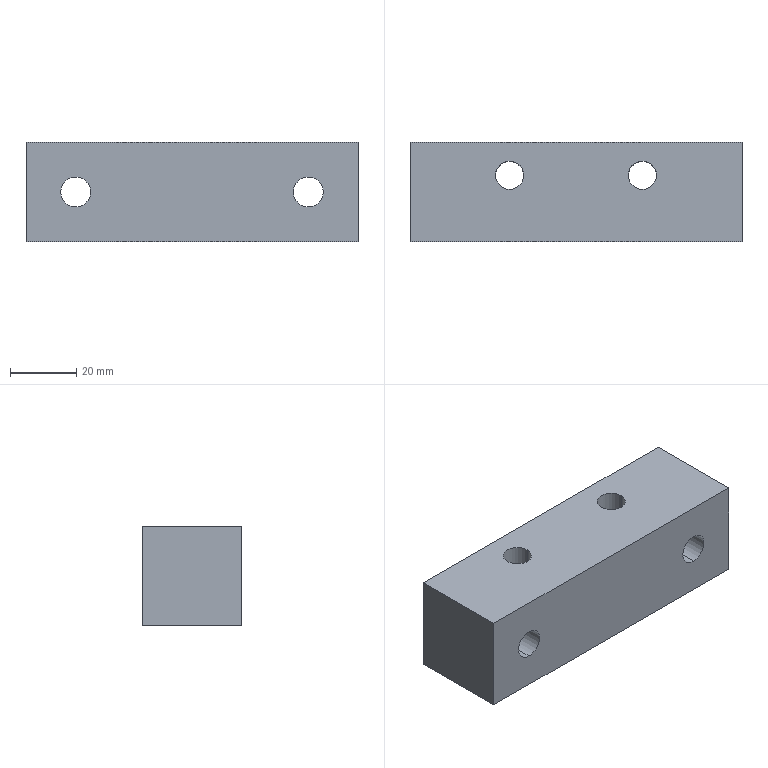Part | SolidWorks | features HoleWzd 2, Extrusion 1 | 1 solid | 20 faces | box 100 x 30 x 30 mm | volume 78254 mm3 | cylinder 12 | plane 8 | commonest cylinder face diameters 8.5 x4 9 x4 15 x4
STEP:
#1=CARTESIAN_POINT('',(-24.25,5.,0.));
#2=VERTEX_POINT('',#1);
#3=CARTESIAN_POINT('',(-15.75,5.,0.));
#4=VERTEX_POINT('',#3);
#5=CARTESIAN_POINT('',(-20.,5.,0.));
#6=DIRECTION('',(0.,0.,1.));
#7=DIRECTION('',(1.,0.,0.));
#8=AXIS2_PLACEMENT_3D('',#5,#6,#7);
#9=CIRCLE('',#8,4.25);
#10=EDGE_CURVE('',#2,#4,#9,.T.);
#11=ORIENTED_EDGE('',*,*,#10,.F.);
#12=CARTESIAN_POINT('',(-24.25,5.,30.));
#13=VERTEX_POINT('',#12);
#14=CARTESIAN_POINT('',(-24.25,5.,30.));
#15=DIRECTION('',(0.,0.,1.));
#16=VECTOR('',#15,1000.);
#17=LINE('',#14,#16);
#18=EDGE_CURVE('',#2,#13,#17,.T.);
#19=ORIENTED_EDGE('',*,*,#18,.T.);
#20=CARTESIAN_POINT('',(-15.75,5.,30.));
#21=VERTEX_POINT('',#20);
#22=CARTESIAN_POINT('',(-20.,5.,30.));
#23=DIRECTION('',(0.,0.,1.));
#24=DIRECTION('',(1.,0.,0.));
#25=AXIS2_PLACEMENT_3D('',#22,#23,#24);
#26=CIRCLE('',#25,4.25);
#27=EDGE_CURVE('',#13,#21,#26,.T.);
#28=ORIENTED_EDGE('',*,*,#27,.T.);
#29=CARTESIAN_POINT('',(-15.75,5.,30.));
#30=DIRECTION('',(0.,0.,1.));
#31=VECTOR('',#30,1000.);
#32=LINE('',#29,#31);
#33=EDGE_CURVE('',#4,#21,#32,.T.);
#34=ORIENTED_EDGE('',*,*,#33,.F.);
#35=EDGE_LOOP('',(#11,#19,#28,#34));
#36=FACE_OUTER_BOUND('',#35,.T.);
#37=CARTESIAN_POINT('',(-20.,5.,30.));
#38=DIRECTION('',(0.,0.,1.));
#39=DIRECTION('',(1.,0.,0.));
#40=AXIS2_PLACEMENT_3D('',#37,#38,#39);
#41=CYLINDRICAL_SURFACE('',#40,4.25);
#42=ADVANCED_FACE('',(#36),#41,.F.);
#43=CARTESIAN_POINT('',(15.75,5.,0.));
#44=VERTEX_POINT('',#43);
#45=CARTESIAN_POINT('',(24.25,5.,0.));
#46=VERTEX_POINT('',#45);
#47=CARTESIAN_POINT('',(20.,5.,0.));
#48=DIRECTION('',(0.,0.,1.));
#49=DIRECTION('',(1.,0.,0.));
#50=AXIS2_PLACEMENT_3D('',#47,#48,#49);
#51=CIRCLE('',#50,4.25);
#52=EDGE_CURVE('',#44,#46,#51,.T.);
#53=ORIENTED_EDGE('',*,*,#52,.F.);
#54=CARTESIAN_POINT('',(15.75,5.,30.));
#55=VERTEX_POINT('',#54);
#56=CARTESIAN_POINT('',(15.75,5.,30.));
#57=DIRECTION('',(0.,0.,1.));
#58=VECTOR('',#57,1000.);
#59=LINE('',#56,#58);
#60=EDGE_CURVE('',#44,#55,#59,.T.);
#61=ORIENTED_EDGE('',*,*,#60,.T.);
#62=CARTESIAN_POINT('',(24.25,5.,30.));
#63=VERTEX_POINT('',#62);
#64=CARTESIAN_POINT('',(20.,5.,30.));
#65=DIRECTION('',(0.,0.,1.));
#66=DIRECTION('',(1.,0.,0.));
#67=AXIS2_PLACEMENT_3D('',#64,#65,#66);
#68=CIRCLE('',#67,4.25);
#69=EDGE_CURVE('',#55,#63,#68,.T.);
#70=ORIENTED_EDGE('',*,*,#69,.T.);
#71=CARTESIAN_POINT('',(24.25,5.,30.));
#72=DIRECTION('',(0.,0.,1.));
#73=VECTOR('',#72,1000.);
#74=LINE('',#71,#73);
#75=EDGE_CURVE('',#46,#63,#74,.T.);
#76=ORIENTED_EDGE('',*,*,#75,.F.);
#77=EDGE_LOOP('',(#53,#61,#70,#76));
#78=FACE_OUTER_BOUND('',#77,.T.);
#79=CARTESIAN_POINT('',(20.,5.,30.));
#80=DIRECTION('',(0.,0.,1.));
#81=DIRECTION('',(1.,0.,0.));
#82=AXIS2_PLACEMENT_3D('',#79,#80,#81);
#83=CYLINDRICAL_SURFACE('',#82,4.25);
#84=ADVANCED_FACE('',(#78),#83,.F.);
#85=CARTESIAN_POINT('',(-35.,-5.,7.5));
#86=VERTEX_POINT('',#85);
#87=CARTESIAN_POINT('',(-35.,-5.,22.5));
#88=VERTEX_POINT('',#87);
#89=CARTESIAN_POINT('',(-35.,-5.,15.));
#90=DIRECTION('',(0.,1.,0.));
#91=DIRECTION('',(0.,0.,1.));
#92=AXIS2_PLACEMENT_3D('',#89,#90,#91);
#93=CIRCLE('',#92,7.5);
#94=EDGE_CURVE('',#86,#88,#93,.T.);
#95=ORIENTED_EDGE('',*,*,#94,.F.);
#96=CARTESIAN_POINT('',(-35.,15.,7.5));
#97=VERTEX_POINT('',#96);
#98=CARTESIAN_POINT('',(-35.,15.,7.5));
#99=DIRECTION('',(0.,1.,0.));
#100=VECTOR('',#99,1000.);
#101=LINE('',#98,#100);
#102=EDGE_CURVE('',#86,#97,#101,.T.);
#103=ORIENTED_EDGE('',*,*,#102,.T.);
#104=CARTESIAN_POINT('',(-35.,15.,22.5));
#105=VERTEX_POINT('',#104);
#106=CARTESIAN_POINT('',(-35.,15.,15.));
#107=DIRECTION('',(0.,1.,0.));
#108=DIRECTION('',(0.,0.,1.));
#109=AXIS2_PLACEMENT_3D('',#106,#107,#108);
#110=CIRCLE('',#109,7.5);
#111=EDGE_CURVE('',#97,#105,#110,.T.);
#112=ORIENTED_EDGE('',*,*,#111,.T.);
#113=CARTESIAN_POINT('',(-35.,15.,22.5));
#114=DIRECTION('',(0.,1.,0.));
#115=VECTOR('',#114,1000.);
#116=LINE('',#113,#115);
#117=EDGE_CURVE('',#88,#105,#116,.T.);
#118=ORIENTED_EDGE('',*,*,#117,.F.);
#119=EDGE_LOOP('',(#95,#103,#112,#118));
#120=FACE_OUTER_BOUND('',#119,.T.);
#121=CARTESIAN_POINT('',(-35.,15.,15.));
#122=DIRECTION('',(0.,1.,0.));
#123=DIRECTION('',(0.,0.,1.));
#124=AXIS2_PLACEMENT_3D('',#121,#122,#123);
#125=CYLINDRICAL_SURFACE('',#124,7.5);
#126=ADVANCED_FACE('',(#120),#125,.F.);
#127=CARTESIAN_POINT('',(-35.,-15.,10.5));
#128=VERTEX_POINT('',#127);
#129=CARTESIAN_POINT('',(-35.,-15.,19.5));
#130=VERTEX_POINT('',#129);
#131=CARTESIAN_POINT('',(-35.,-15.,15.));
#132=DIRECTION('',(0.,1.,0.));
#133=DIRECTION('',(0.,0.,1.));
#134=AXIS2_PLACEMENT_3D('',#131,#132,#133);
#135=CIRCLE('',#134,4.5);
#136=EDGE_CURVE('',#128,#130,#135,.T.);
#137=ORIENTED_EDGE('',*,*,#136,.F.);
#138=CARTESIAN_POINT('',(-35.,-5.,10.5));
#139=VERTEX_POINT('',#138);
#140=CARTESIAN_POINT('',(-35.,15.,10.5));
#141=DIRECTION('',(0.,1.,0.));
#142=VECTOR('',#141,1000.);
#143=LINE('',#140,#142);
#144=EDGE_CURVE('',#128,#139,#143,.T.);
#145=ORIENTED_EDGE('',*,*,#144,.T.);
#146=CARTESIAN_POINT('',(-35.,-5.,19.5));
#147=VERTEX_POINT('',#146);
#148=CARTESIAN_POINT('',(-35.,-5.,15.));
#149=DIRECTION('',(0.,1.,0.));
#150=DIRECTION('',(0.,0.,1.));
#151=AXIS2_PLACEMENT_3D('',#148,#149,#150);
#152=CIRCLE('',#151,4.5);
#153=EDGE_CURVE('',#139,#147,#152,.T.);
#154=ORIENTED_EDGE('',*,*,#153,.T.);
#155=CARTESIAN_POINT('',(-35.,15.,19.5));
#156=DIRECTION('',(0.,1.,0.));
#157=VECTOR('',#156,1000.);
#158=LINE('',#155,#157);
#159=EDGE_CURVE('',#130,#147,#158,.T.);
#160=ORIENTED_EDGE('',*,*,#159,.F.);
#161=EDGE_LOOP('',(#137,#145,#154,#160));
#162=FACE_OUTER_BOUND('',#161,.T.);
#163=CARTESIAN_POINT('',(-35.,15.,15.));
#164=DIRECTION('',(0.,1.,0.));
#165=DIRECTION('',(0.,0.,1.));
#166=AXIS2_PLACEMENT_3D('',#163,#164,#165);
#167=CYLINDRICAL_SURFACE('',#166,4.5);
#168=ADVANCED_FACE('',(#162),#167,.F.);
#169=CARTESIAN_POINT('',(35.,-5.,7.5));
#170=VERTEX_POINT('',#169);
#171=CARTESIAN_POINT('',(35.,-5.,22.5));
#172=VERTEX_POINT('',#171);
#173=CARTESIAN_POINT('',(35.,-5.,15.));
#174=DIRECTION('',(0.,1.,0.));
#175=DIRECTION('',(0.,0.,1.));
#176=AXIS2_PLACEMENT_3D('',#173,#174,#175);
#177=CIRCLE('',#176,7.5);
#178=EDGE_CURVE('',#170,#172,#177,.T.);
#179=ORIENTED_EDGE('',*,*,#178,.F.);
#180=CARTESIAN_POINT('',(35.,15.,7.5));
#181=VERTEX_POINT('',#180);
#182=CARTESIAN_POINT('',(35.,15.,7.5));
#183=DIRECTION('',(0.,1.,0.));
#184=VECTOR('',#183,1000.);
#185=LINE('',#182,#184);
#186=EDGE_CURVE('',#170,#181,#185,.T.);
#187=ORIENTED_EDGE('',*,*,#186,.T.);
#188=CARTESIAN_POINT('',(35.,15.,22.5));
#189=VERTEX_POINT('',#188);
#190=CARTESIAN_POINT('',(35.,15.,15.));
#191=DIRECTION('',(0.,1.,0.));
#192=DIRECTION('',(0.,0.,1.));
#193=AXIS2_PLACEMENT_3D('',#190,#191,#192);
#194=CIRCLE('',#193,7.5);
#195=EDGE_CURVE('',#181,#189,#194,.T.);
#196=ORIENTED_EDGE('',*,*,#195,.T.);
#197=CARTESIAN_POINT('',(35.,15.,22.5));
#198=DIRECTION('',(0.,1.,0.));
#199=VECTOR('',#198,1000.);
#200=LINE('',#197,#199);
#201=EDGE_CURVE('',#172,#189,#200,.T.);
#202=ORIENTED_EDGE('',*,*,#201,.F.);
#203=EDGE_LOOP('',(#179,#187,#196,#202));
#204=FACE_OUTER_BOUND('',#203,.T.);
#205=CARTESIAN_POINT('',(35.,15.,15.));
#206=DIRECTION('',(0.,1.,0.));
#207=DIRECTION('',(0.,0.,1.));
#208=AXIS2_PLACEMENT_3D('',#205,#206,#207);
#209=CYLINDRICAL_SURFACE('',#208,7.5);
#210=ADVANCED_FACE('',(#204),#209,.F.);
#211=CARTESIAN_POINT('',(35.,-15.,10.5));
#212=VERTEX_POINT('',#211);
#213=CARTESIAN_POINT('',(35.,-15.,19.5));
#214=VERTEX_POINT('',#213);
#215=CARTESIAN_POINT('',(35.,-15.,15.));
#216=DIRECTION('',(0.,1.,0.));
#217=DIRECTION('',(0.,0.,1.));
#218=AXIS2_PLACEMENT_3D('',#215,#216,#217);
#219=CIRCLE('',#218,4.5);
#220=EDGE_CURVE('',#212,#214,#219,.T.);
#221=ORIENTED_EDGE('',*,*,#220,.F.);
#222=CARTESIAN_POINT('',(35.,-5.,10.5));
#223=VERTEX_POINT('',#222);
#224=CARTESIAN_POINT('',(35.,15.,10.5));
#225=DIRECTION('',(0.,1.,0.));
#226=VECTOR('',#225,1000.);
#227=LINE('',#224,#226);
#228=EDGE_CURVE('',#212,#223,#227,.T.);
#229=ORIENTED_EDGE('',*,*,#228,.T.);
#230=CARTESIAN_POINT('',(35.,-5.,19.5));
#231=VERTEX_POINT('',#230);
#232=CARTESIAN_POINT('',(35.,-5.,15.));
#233=DIRECTION('',(0.,1.,0.));
#234=DIRECTION('',(0.,0.,1.));
#235=AXIS2_PLACEMENT_3D('',#232,#233,#234);
#236=CIRCLE('',#235,4.5);
#237=EDGE_CURVE('',#223,#231,#236,.T.);
#238=ORIENTED_EDGE('',*,*,#237,.T.);
#239=CARTESIAN_POINT('',(35.,15.,19.5));
#240=DIRECTION('',(0.,1.,0.));
#241=VECTOR('',#240,1000.);
#242=LINE('',#239,#241);
#243=EDGE_CURVE('',#214,#231,#242,.T.);
#244=ORIENTED_EDGE('',*,*,#243,.F.);
#245=EDGE_LOOP('',(#221,#229,#238,#244));
#246=FACE_OUTER_BOUND('',#245,.T.);
#247=CARTESIAN_POINT('',(35.,15.,15.));
#248=DIRECTION('',(0.,1.,0.));
#249=DIRECTION('',(0.,0.,1.));
#250=AXIS2_PLACEMENT_3D('',#247,#248,#249);
#251=CYLINDRICAL_SURFACE('',#250,4.5);
#252=ADVANCED_FACE('',(#246),#251,.F.);
#253=CARTESIAN_POINT('',(-35.,15.,15.));
#254=DIRECTION('',(0.,1.,0.));
#255=DIRECTION('',(0.,0.,1.));
#256=AXIS2_PLACEMENT_3D('',#253,#254,#255);
#257=CIRCLE('',#256,7.5);
#258=EDGE_CURVE('',#105,#97,#257,.T.);
#259=ORIENTED_EDGE('',*,*,#258,.F.);
#260=ORIENTED_EDGE('',*,*,#111,.F.);
#261=EDGE_LOOP('',(#259,#260));
#262=FACE_BOUND('',#261,.T.);
#263=CARTESIAN_POINT('',(50.,15.,0.));
#264=VERTEX_POINT('',#263);
#265=CARTESIAN_POINT('',(-50.,15.,0.));
#266=VERTEX_POINT('',#265);
#267=CARTESIAN_POINT('',(-50.,15.,0.));
#268=DIRECTION('',(-1.,0.,0.));
#269=VECTOR('',#268,1000.);
#270=LINE('',#267,#269);
#271=EDGE_CURVE('',#264,#266,#270,.T.);
#272=ORIENTED_EDGE('',*,*,#271,.T.);
#273=CARTESIAN_POINT('',(-50.,15.,30.));
#274=VERTEX_POINT('',#273);
#275=CARTESIAN_POINT('',(-50.,15.,30.));
#276=DIRECTION('',(0.,0.,-1.));
#277=VECTOR('',#276,1000.);
#278=LINE('',#275,#277);
#279=EDGE_CURVE('',#274,#266,#278,.T.);
#280=ORIENTED_EDGE('',*,*,#279,.F.);
#281=CARTESIAN_POINT('',(50.,15.,30.));
#282=VERTEX_POINT('',#281);
#283=CARTESIAN_POINT('',(-50.,15.,30.));
#284=DIRECTION('',(-1.,0.,0.));
#285=VECTOR('',#284,1000.);
#286=LINE('',#283,#285);
#287=EDGE_CURVE('',#282,#274,#286,.T.);
#288=ORIENTED_EDGE('',*,*,#287,.F.);
#289=CARTESIAN_POINT('',(50.,15.,30.));
#290=DIRECTION('',(0.,0.,-1.));
#291=VECTOR('',#290,1000.);
#292=LINE('',#289,#291);
#293=EDGE_CURVE('',#282,#264,#292,.T.);
#294=ORIENTED_EDGE('',*,*,#293,.T.);
#295=EDGE_LOOP('',(#272,#280,#288,#294));
#296=FACE_OUTER_BOUND('',#295,.T.);
#297=CARTESIAN_POINT('',(35.,15.,15.));
#298=DIRECTION('',(0.,1.,0.));
#299=DIRECTION('',(0.,0.,1.));
#300=AXIS2_PLACEMENT_3D('',#297,#298,#299);
#301=CIRCLE('',#300,7.5);
#302=EDGE_CURVE('',#189,#181,#301,.T.);
#303=ORIENTED_EDGE('',*,*,#302,.F.);
#304=ORIENTED_EDGE('',*,*,#195,.F.);
#305=EDGE_LOOP('',(#303,#304));
#306=FACE_BOUND('',#305,.T.);
#307=CARTESIAN_POINT('',(-50.,15.,30.));
#308=DIRECTION('',(0.,-1.,0.));
#309=DIRECTION('',(0.,0.,-1.));
#310=AXIS2_PLACEMENT_3D('',#307,#308,#309);
#311=PLANE('',#310);
#312=ADVANCED_FACE('',(#262,#296,#306),#311,.F.);
#313=CARTESIAN_POINT('',(50.,-15.,0.));
#314=VERTEX_POINT('',#313);
#315=CARTESIAN_POINT('',(50.,15.,0.));
#316=DIRECTION('',(0.,1.,0.));
#317=VECTOR('',#316,1000.);
#318=LINE('',#315,#317);
#319=EDGE_CURVE('',#314,#264,#318,.T.);
#320=ORIENTED_EDGE('',*,*,#319,.T.);
#321=ORIENTED_EDGE('',*,*,#293,.F.);
#322=CARTESIAN_POINT('',(50.,-15.,30.));
#323=VERTEX_POINT('',#322);
#324=CARTESIAN_POINT('',(50.,15.,30.));
#325=DIRECTION('',(0.,1.,0.));
#326=VECTOR('',#325,1000.);
#327=LINE('',#324,#326);
#328=EDGE_CURVE('',#323,#282,#327,.T.);
#329=ORIENTED_EDGE('',*,*,#328,.F.);
#330=CARTESIAN_POINT('',(50.,-15.,30.));
#331=DIRECTION('',(0.,0.,-1.));
#332=VECTOR('',#331,1000.);
#333=LINE('',#330,#332);
#334=EDGE_CURVE('',#323,#314,#333,.T.);
#335=ORIENTED_EDGE('',*,*,#334,.T.);
#336=EDGE_LOOP('',(#320,#321,#329,#335));
#337=FACE_OUTER_BOUND('',#336,.T.);
#338=CARTESIAN_POINT('',(50.,15.,30.));
#339=DIRECTION('',(-1.,0.,0.));
#340=DIRECTION('',(0.,-1.,0.));
#341=AXIS2_PLACEMENT_3D('',#338,#339,#340);
#342=PLANE('',#341);
#343=ADVANCED_FACE('',(#337),#342,.F.);
#344=CARTESIAN_POINT('',(-50.,-15.,0.));
#345=VERTEX_POINT('',#344);
#346=CARTESIAN_POINT('',(-50.,15.,0.));
#347=DIRECTION('',(0.,-1.,0.));
#348=VECTOR('',#347,1000.);
#349=LINE('',#346,#348);
#350=EDGE_CURVE('',#266,#345,#349,.T.);
#351=ORIENTED_EDGE('',*,*,#350,.T.);
#352=CARTESIAN_POINT('',(-50.,-15.,30.));
#353=VERTEX_POINT('',#352);
#354=CARTESIAN_POINT('',(-50.,-15.,30.));
#355=DIRECTION('',(0.,0.,-1.));
#356=VECTOR('',#355,1000.);
#357=LINE('',#354,#356);
#358=EDGE_CURVE('',#353,#345,#357,.T.);
#359=ORIENTED_EDGE('',*,*,#358,.F.);
#360=CARTESIAN_POINT('',(-50.,15.,30.));
#361=DIRECTION('',(0.,-1.,0.));
#362=VECTOR('',#361,1000.);
#363=LINE('',#360,#362);
#364=EDGE_CURVE('',#274,#353,#363,.T.);
#365=ORIENTED_EDGE('',*,*,#364,.F.);
#366=ORIENTED_EDGE('',*,*,#279,.T.);
#367=EDGE_LOOP('',(#351,#359,#365,#366));
#368=FACE_OUTER_BOUND('',#367,.T.);
#369=CARTESIAN_POINT('',(-50.,15.,30.));
#370=DIRECTION('',(1.,0.,0.));
#371=DIRECTION('',(0.,1.,0.));
#372=AXIS2_PLACEMENT_3D('',#369,#370,#371);
#373=PLANE('',#372);
#374=ADVANCED_FACE('',(#368),#373,.F.);
#375=CARTESIAN_POINT('',(-35.,-15.,15.));
#376=DIRECTION('',(0.,1.,0.));
#377=DIRECTION('',(0.,0.,1.));
#378=AXIS2_PLACEMENT_3D('',#375,#376,#377);
#379=CIRCLE('',#378,4.5);
#380=EDGE_CURVE('',#130,#128,#379,.T.);
#381=ORIENTED_EDGE('',*,*,#380,.T.);
#382=ORIENTED_EDGE('',*,*,#136,.T.);
#383=EDGE_LOOP('',(#381,#382));
#384=FACE_BOUND('',#383,.T.);
#385=CARTESIAN_POINT('',(35.,-15.,15.));
#386=DIRECTION('',(0.,1.,0.));
#387=DIRECTION('',(0.,0.,1.));
#388=AXIS2_PLACEMENT_3D('',#385,#386,#387);
#389=CIRCLE('',#388,4.5);
#390=EDGE_CURVE('',#214,#212,#389,.T.);
#391=ORIENTED_EDGE('',*,*,#390,.T.);
#392=ORIENTED_EDGE('',*,*,#220,.T.);
#393=EDGE_LOOP('',(#391,#392));
#394=FACE_BOUND('',#393,.T.);
#395=CARTESIAN_POINT('',(-50.,-15.,0.));
#396=DIRECTION('',(1.,0.,0.));
#397=VECTOR('',#396,1000.);
#398=LINE('',#395,#397);
#399=EDGE_CURVE('',#345,#314,#398,.T.);
#400=ORIENTED_EDGE('',*,*,#399,.T.);
#401=ORIENTED_EDGE('',*,*,#334,.F.);
#402=CARTESIAN_POINT('',(-50.,-15.,30.));
#403=DIRECTION('',(1.,0.,0.));
#404=VECTOR('',#403,1000.);
#405=LINE('',#402,#404);
#406=EDGE_CURVE('',#353,#323,#405,.T.);
#407=ORIENTED_EDGE('',*,*,#406,.F.);
#408=ORIENTED_EDGE('',*,*,#358,.T.);
#409=EDGE_LOOP('',(#400,#401,#407,#408));
#410=FACE_OUTER_BOUND('',#409,.T.);
#411=CARTESIAN_POINT('',(-50.,-15.,30.));
#412=DIRECTION('',(0.,1.,0.));
#413=DIRECTION('',(0.,0.,1.));
#414=AXIS2_PLACEMENT_3D('',#411,#412,#413);
#415=PLANE('',#414);
#416=ADVANCED_FACE('',(#384,#394,#410),#415,.F.);
#417=CARTESIAN_POINT('',(-20.,5.,30.));
#418=DIRECTION('',(0.,0.,1.));
#419=DIRECTION('',(1.,0.,0.));
#420=AXIS2_PLACEMENT_3D('',#417,#418,#419);
#421=CIRCLE('',#420,4.25);
#422=EDGE_CURVE('',#21,#13,#421,.T.);
#423=ORIENTED_EDGE('',*,*,#422,.F.);
#424=ORIENTED_EDGE('',*,*,#27,.F.);
#425=EDGE_LOOP('',(#423,#424));
#426=FACE_BOUND('',#425,.T.);
#427=CARTESIAN_POINT('',(20.,5.,30.));
#428=DIRECTION('',(0.,0.,1.));
#429=DIRECTION('',(1.,0.,0.));
#430=AXIS2_PLACEMENT_3D('',#427,#428,#429);
#431=CIRCLE('',#430,4.25);
#432=EDGE_CURVE('',#63,#55,#431,.T.);
#433=ORIENTED_EDGE('',*,*,#432,.F.);
#434=ORIENTED_EDGE('',*,*,#69,.F.);
#435=EDGE_LOOP('',(#433,#434));
#436=FACE_BOUND('',#435,.T.);
#437=ORIENTED_EDGE('',*,*,#328,.T.);
#438=ORIENTED_EDGE('',*,*,#287,.T.);
#439=ORIENTED_EDGE('',*,*,#364,.T.);
#440=ORIENTED_EDGE('',*,*,#406,.T.);
#441=EDGE_LOOP('',(#437,#438,#439,#440));
#442=FACE_OUTER_BOUND('',#441,.T.);
#443=CARTESIAN_POINT('',(0.,0.,30.));
#444=DIRECTION('',(0.,0.,1.));
#445=DIRECTION('',(1.,0.,0.));
#446=AXIS2_PLACEMENT_3D('',#443,#444,#445);
#447=PLANE('',#446);
#448=ADVANCED_FACE('',(#426,#436,#442),#447,.T.);
#449=CARTESIAN_POINT('',(-20.,5.,0.));
#450=DIRECTION('',(0.,0.,1.));
#451=DIRECTION('',(1.,0.,0.));
#452=AXIS2_PLACEMENT_3D('',#449,#450,#451);
#453=CIRCLE('',#452,4.25);
#454=EDGE_CURVE('',#4,#2,#453,.T.);
#455=ORIENTED_EDGE('',*,*,#454,.T.);
#456=ORIENTED_EDGE('',*,*,#10,.T.);
#457=EDGE_LOOP('',(#455,#456));
#458=FACE_BOUND('',#457,.T.);
#459=CARTESIAN_POINT('',(20.,5.,0.));
#460=DIRECTION('',(0.,0.,1.));
#461=DIRECTION('',(1.,0.,0.));
#462=AXIS2_PLACEMENT_3D('',#459,#460,#461);
#463=CIRCLE('',#462,4.25);
#464=EDGE_CURVE('',#46,#44,#463,.T.);
#465=ORIENTED_EDGE('',*,*,#464,.T.);
#466=ORIENTED_EDGE('',*,*,#52,.T.);
#467=EDGE_LOOP('',(#465,#466));
#468=FACE_BOUND('',#467,.T.);
#469=ORIENTED_EDGE('',*,*,#319,.F.);
#470=ORIENTED_EDGE('',*,*,#399,.F.);
#471=ORIENTED_EDGE('',*,*,#350,.F.);
#472=ORIENTED_EDGE('',*,*,#271,.F.);
#473=EDGE_LOOP('',(#469,#470,#471,#472));
#474=FACE_OUTER_BOUND('',#473,.T.);
#475=CARTESIAN_POINT('',(0.,0.,0.));
#476=DIRECTION('',(0.,0.,1.));
#477=DIRECTION('',(1.,0.,0.));
#478=AXIS2_PLACEMENT_3D('',#475,#476,#477);
#479=PLANE('',#478);
#480=ADVANCED_FACE('',(#458,#468,#474),#479,.F.);
#481=ORIENTED_EDGE('',*,*,#228,.F.);
#482=ORIENTED_EDGE('',*,*,#390,.F.);
#483=ORIENTED_EDGE('',*,*,#243,.T.);
#484=CARTESIAN_POINT('',(35.,-5.,15.));
#485=DIRECTION('',(0.,1.,0.));
#486=DIRECTION('',(0.,0.,1.));
#487=AXIS2_PLACEMENT_3D('',#484,#485,#486);
#488=CIRCLE('',#487,4.5);
#489=EDGE_CURVE('',#231,#223,#488,.T.);
#490=ORIENTED_EDGE('',*,*,#489,.T.);
#491=EDGE_LOOP('',(#481,#482,#483,#490));
#492=FACE_OUTER_BOUND('',#491,.T.);
#493=CARTESIAN_POINT('',(35.,15.,15.));
#494=DIRECTION('',(0.,1.,0.));
#495=DIRECTION('',(0.,0.,1.));
#496=AXIS2_PLACEMENT_3D('',#493,#494,#495);
#497=CYLINDRICAL_SURFACE('',#496,4.5);
#498=ADVANCED_FACE('',(#492),#497,.F.);
#499=ORIENTED_EDGE('',*,*,#489,.F.);
#500=ORIENTED_EDGE('',*,*,#237,.F.);
#501=EDGE_LOOP('',(#499,#500));
#502=FACE_BOUND('',#501,.T.);
#503=CARTESIAN_POINT('',(35.,-5.,15.));
#504=DIRECTION('',(0.,1.,0.));
#505=DIRECTION('',(0.,0.,1.));
#506=AXIS2_PLACEMENT_3D('',#503,#504,#505);
#507=CIRCLE('',#506,7.5);
#508=EDGE_CURVE('',#172,#170,#507,.T.);
#509=ORIENTED_EDGE('',*,*,#508,.T.);
#510=ORIENTED_EDGE('',*,*,#178,.T.);
#511=EDGE_LOOP('',(#509,#510));
#512=FACE_OUTER_BOUND('',#511,.T.);
#513=CARTESIAN_POINT('',(39.5,-5.,15.));
#514=DIRECTION('',(0.,-1.,0.));
#515=DIRECTION('',(0.,0.,-1.));
#516=AXIS2_PLACEMENT_3D('',#513,#514,#515);
#517=PLANE('',#516);
#518=ADVANCED_FACE('',(#502,#512),#517,.F.);
#519=ORIENTED_EDGE('',*,*,#186,.F.);
#520=ORIENTED_EDGE('',*,*,#508,.F.);
#521=ORIENTED_EDGE('',*,*,#201,.T.);
#522=ORIENTED_EDGE('',*,*,#302,.T.);
#523=EDGE_LOOP('',(#519,#520,#521,#522));
#524=FACE_OUTER_BOUND('',#523,.T.);
#525=CARTESIAN_POINT('',(35.,15.,15.));
#526=DIRECTION('',(0.,1.,0.));
#527=DIRECTION('',(0.,0.,1.));
#528=AXIS2_PLACEMENT_3D('',#525,#526,#527);
#529=CYLINDRICAL_SURFACE('',#528,7.5);
#530=ADVANCED_FACE('',(#524),#529,.F.);
#531=ORIENTED_EDGE('',*,*,#144,.F.);
#532=ORIENTED_EDGE('',*,*,#380,.F.);
#533=ORIENTED_EDGE('',*,*,#159,.T.);
#534=CARTESIAN_POINT('',(-35.,-5.,15.));
#535=DIRECTION('',(0.,1.,0.));
#536=DIRECTION('',(0.,0.,1.));
#537=AXIS2_PLACEMENT_3D('',#534,#535,#536);
#538=CIRCLE('',#537,4.5);
#539=EDGE_CURVE('',#147,#139,#538,.T.);
#540=ORIENTED_EDGE('',*,*,#539,.T.);
#541=EDGE_LOOP('',(#531,#532,#533,#540));
#542=FACE_OUTER_BOUND('',#541,.T.);
#543=CARTESIAN_POINT('',(-35.,15.,15.));
#544=DIRECTION('',(0.,1.,0.));
#545=DIRECTION('',(0.,0.,1.));
#546=AXIS2_PLACEMENT_3D('',#543,#544,#545);
#547=CYLINDRICAL_SURFACE('',#546,4.5);
#548=ADVANCED_FACE('',(#542),#547,.F.);
#549=ORIENTED_EDGE('',*,*,#539,.F.);
#550=ORIENTED_EDGE('',*,*,#153,.F.);
#551=EDGE_LOOP('',(#549,#550));
#552=FACE_BOUND('',#551,.T.);
#553=CARTESIAN_POINT('',(-35.,-5.,15.));
#554=DIRECTION('',(0.,1.,0.));
#555=DIRECTION('',(0.,0.,1.));
#556=AXIS2_PLACEMENT_3D('',#553,#554,#555);
#557=CIRCLE('',#556,7.5);
#558=EDGE_CURVE('',#88,#86,#557,.T.);
#559=ORIENTED_EDGE('',*,*,#558,.T.);
#560=ORIENTED_EDGE('',*,*,#94,.T.);
#561=EDGE_LOOP('',(#559,#560));
#562=FACE_OUTER_BOUND('',#561,.T.);
#563=CARTESIAN_POINT('',(-30.5,-5.,15.));
#564=DIRECTION('',(0.,-1.,0.));
#565=DIRECTION('',(0.,0.,-1.));
#566=AXIS2_PLACEMENT_3D('',#563,#564,#565);
#567=PLANE('',#566);
#568=ADVANCED_FACE('',(#552,#562),#567,.F.);
#569=ORIENTED_EDGE('',*,*,#102,.F.);
#570=ORIENTED_EDGE('',*,*,#558,.F.);
#571=ORIENTED_EDGE('',*,*,#117,.T.);
#572=ORIENTED_EDGE('',*,*,#258,.T.);
#573=EDGE_LOOP('',(#569,#570,#571,#572));
#574=FACE_OUTER_BOUND('',#573,.T.);
#575=CARTESIAN_POINT('',(-35.,15.,15.));
#576=DIRECTION('',(0.,1.,0.));
#577=DIRECTION('',(0.,0.,1.));
#578=AXIS2_PLACEMENT_3D('',#575,#576,#577);
#579=CYLINDRICAL_SURFACE('',#578,7.5);
#580=ADVANCED_FACE('',(#574),#579,.F.);
#581=ORIENTED_EDGE('',*,*,#60,.F.);
#582=ORIENTED_EDGE('',*,*,#464,.F.);
#583=ORIENTED_EDGE('',*,*,#75,.T.);
#584=ORIENTED_EDGE('',*,*,#432,.T.);
#585=EDGE_LOOP('',(#581,#582,#583,#584));
#586=FACE_OUTER_BOUND('',#585,.T.);
#587=CARTESIAN_POINT('',(20.,5.,30.));
#588=DIRECTION('',(0.,0.,1.));
#589=DIRECTION('',(1.,0.,0.));
#590=AXIS2_PLACEMENT_3D('',#587,#588,#589);
#591=CYLINDRICAL_SURFACE('',#590,4.25);
#592=ADVANCED_FACE('',(#586),#591,.F.);
#593=ORIENTED_EDGE('',*,*,#18,.F.);
#594=ORIENTED_EDGE('',*,*,#454,.F.);
#595=ORIENTED_EDGE('',*,*,#33,.T.);
#596=ORIENTED_EDGE('',*,*,#422,.T.);
#597=EDGE_LOOP('',(#593,#594,#595,#596));
#598=FACE_OUTER_BOUND('',#597,.T.);
#599=CARTESIAN_POINT('',(-20.,5.,30.));
#600=DIRECTION('',(0.,0.,1.));
#601=DIRECTION('',(1.,0.,0.));
#602=AXIS2_PLACEMENT_3D('',#599,#600,#601);
#603=CYLINDRICAL_SURFACE('',#602,4.25);
#604=ADVANCED_FACE('',(#598),#603,.F.);
#605=CLOSED_SHELL('',(#42,#84,#126,#168,#210,#252,#312,#343,#374,#416,#448,#480,#498,#518,#530,#548,#568,#580,#592,#604));
#606=MANIFOLD_SOLID_BREP('',#605);
#607=CARTESIAN_POINT('',(0.,0.,0.));
#608=DIRECTION('',(0.,0.,1.));
#609=DIRECTION('',(1.,0.,0.));
#610=AXIS2_PLACEMENT_3D('',#607,#608,#609);
#611=(LENGTH_UNIT()NAMED_UNIT(*)SI_UNIT(.MILLI.,.METRE.));
#612=UNCERTAINTY_MEASURE_WITH_UNIT(LENGTH_MEASURE(0.00001),#611,'','');
#613=(NAMED_UNIT(*)PLANE_ANGLE_UNIT()SI_UNIT($,.RADIAN.));
#614=(NAMED_UNIT(*)SI_UNIT($,.STERADIAN.)SOLID_ANGLE_UNIT());
#615=(GEOMETRIC_REPRESENTATION_CONTEXT(3)GLOBAL_UNCERTAINTY_ASSIGNED_CONTEXT((#612))GLOBAL_UNIT_ASSIGNED_CONTEXT((#611,#613,#614))REPRESENTATION_CONTEXT('',''));
#616=ADVANCED_BREP_SHAPE_REPRESENTATION('',(#606,#610),#615);